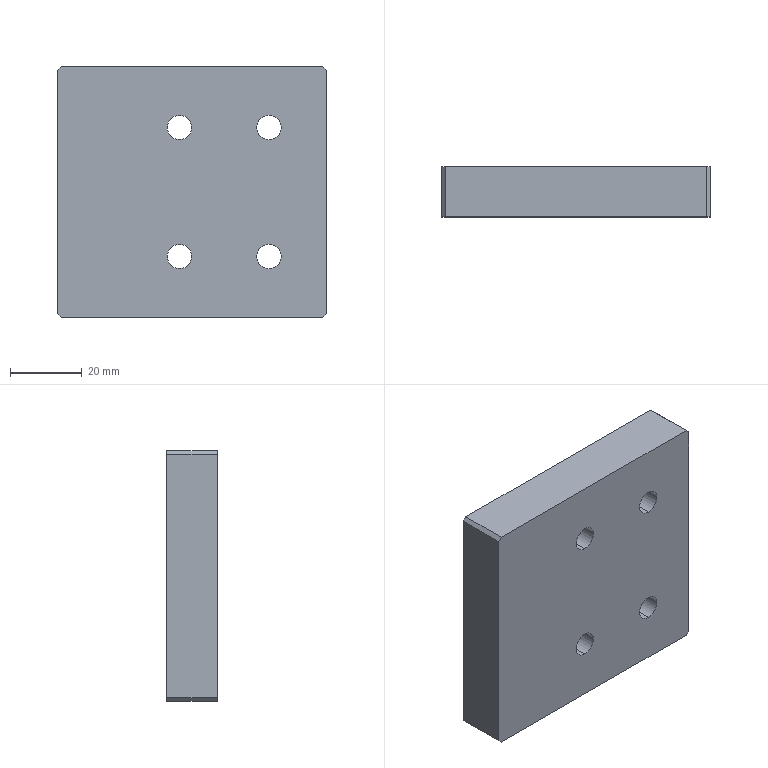Part | SolidWorks | features FlatPattern 1, HoleWzd 1, SMBaseFlange 1, SheetMetal 1 | 1 solid | 18 faces | box 75 x 14 x 70 mm | volume 71438 mm3 | plane 10 | cylinder 8 | commonest cylinder face diameters 6.8 x8
STEP:
#1=CARTESIAN_POINT('',(21.5,0.,-14.6));
#2=VERTEX_POINT('',#1);
#3=CARTESIAN_POINT('',(21.5,0.,-21.4));
#4=VERTEX_POINT('',#3);
#5=CARTESIAN_POINT('',(21.5,0.,-18.));
#6=DIRECTION('',(0.,-1.,0.));
#7=DIRECTION('',(0.,0.,-1.));
#8=AXIS2_PLACEMENT_3D('',#5,#6,#7);
#9=CIRCLE('',#8,3.4);
#10=EDGE_CURVE('',#2,#4,#9,.T.);
#11=ORIENTED_EDGE('',*,*,#10,.T.);
#12=CARTESIAN_POINT('',(21.5,14.,-21.4));
#13=VERTEX_POINT('',#12);
#14=CARTESIAN_POINT('',(21.5,14.,-21.4));
#15=DIRECTION('',(0.,1.,0.));
#16=VECTOR('',#15,1000.);
#17=LINE('',#14,#16);
#18=EDGE_CURVE('',#4,#13,#17,.T.);
#19=ORIENTED_EDGE('',*,*,#18,.T.);
#20=CARTESIAN_POINT('',(21.5,14.,-14.6));
#21=VERTEX_POINT('',#20);
#22=CARTESIAN_POINT('',(21.5,14.,-18.));
#23=DIRECTION('',(0.,1.,0.));
#24=DIRECTION('',(0.,0.,1.));
#25=AXIS2_PLACEMENT_3D('',#22,#23,#24);
#26=CIRCLE('',#25,3.4);
#27=EDGE_CURVE('',#13,#21,#26,.T.);
#28=ORIENTED_EDGE('',*,*,#27,.T.);
#29=CARTESIAN_POINT('',(21.5,14.,-14.6));
#30=DIRECTION('',(0.,1.,0.));
#31=VECTOR('',#30,1000.);
#32=LINE('',#29,#31);
#33=EDGE_CURVE('',#2,#21,#32,.T.);
#34=ORIENTED_EDGE('',*,*,#33,.F.);
#35=EDGE_LOOP('',(#11,#19,#28,#34));
#36=FACE_OUTER_BOUND('',#35,.T.);
#37=CARTESIAN_POINT('',(21.5,14.,-18.));
#38=DIRECTION('',(0.,1.,0.));
#39=DIRECTION('',(0.,0.,1.));
#40=AXIS2_PLACEMENT_3D('',#37,#38,#39);
#41=CYLINDRICAL_SURFACE('',#40,3.4);
#42=ADVANCED_FACE('',(#36),#41,.F.);
#43=CARTESIAN_POINT('',(-3.5,0.,-14.6));
#44=VERTEX_POINT('',#43);
#45=CARTESIAN_POINT('',(-3.5,0.,-21.4));
#46=VERTEX_POINT('',#45);
#47=CARTESIAN_POINT('',(-3.5,0.,-18.));
#48=DIRECTION('',(0.,-1.,0.));
#49=DIRECTION('',(0.,0.,-1.));
#50=AXIS2_PLACEMENT_3D('',#47,#48,#49);
#51=CIRCLE('',#50,3.4);
#52=EDGE_CURVE('',#44,#46,#51,.T.);
#53=ORIENTED_EDGE('',*,*,#52,.T.);
#54=CARTESIAN_POINT('',(-3.5,14.,-21.4));
#55=VERTEX_POINT('',#54);
#56=CARTESIAN_POINT('',(-3.5,14.,-21.4));
#57=DIRECTION('',(0.,1.,0.));
#58=VECTOR('',#57,1000.);
#59=LINE('',#56,#58);
#60=EDGE_CURVE('',#46,#55,#59,.T.);
#61=ORIENTED_EDGE('',*,*,#60,.T.);
#62=CARTESIAN_POINT('',(-3.5,14.,-14.6));
#63=VERTEX_POINT('',#62);
#64=CARTESIAN_POINT('',(-3.5,14.,-18.));
#65=DIRECTION('',(0.,1.,0.));
#66=DIRECTION('',(0.,0.,1.));
#67=AXIS2_PLACEMENT_3D('',#64,#65,#66);
#68=CIRCLE('',#67,3.4);
#69=EDGE_CURVE('',#55,#63,#68,.T.);
#70=ORIENTED_EDGE('',*,*,#69,.T.);
#71=CARTESIAN_POINT('',(-3.5,14.,-14.6));
#72=DIRECTION('',(0.,1.,0.));
#73=VECTOR('',#72,1000.);
#74=LINE('',#71,#73);
#75=EDGE_CURVE('',#44,#63,#74,.T.);
#76=ORIENTED_EDGE('',*,*,#75,.F.);
#77=EDGE_LOOP('',(#53,#61,#70,#76));
#78=FACE_OUTER_BOUND('',#77,.T.);
#79=CARTESIAN_POINT('',(-3.5,14.,-18.));
#80=DIRECTION('',(0.,1.,0.));
#81=DIRECTION('',(0.,0.,1.));
#82=AXIS2_PLACEMENT_3D('',#79,#80,#81);
#83=CYLINDRICAL_SURFACE('',#82,3.4);
#84=ADVANCED_FACE('',(#78),#83,.F.);
#85=CARTESIAN_POINT('',(-3.5,0.,21.4));
#86=VERTEX_POINT('',#85);
#87=CARTESIAN_POINT('',(-3.5,0.,14.6));
#88=VERTEX_POINT('',#87);
#89=CARTESIAN_POINT('',(-3.5,0.,18.));
#90=DIRECTION('',(0.,-1.,0.));
#91=DIRECTION('',(0.,0.,-1.));
#92=AXIS2_PLACEMENT_3D('',#89,#90,#91);
#93=CIRCLE('',#92,3.4);
#94=EDGE_CURVE('',#86,#88,#93,.T.);
#95=ORIENTED_EDGE('',*,*,#94,.T.);
#96=CARTESIAN_POINT('',(-3.5,14.,14.6));
#97=VERTEX_POINT('',#96);
#98=CARTESIAN_POINT('',(-3.5,14.,14.6));
#99=DIRECTION('',(0.,1.,0.));
#100=VECTOR('',#99,1000.);
#101=LINE('',#98,#100);
#102=EDGE_CURVE('',#88,#97,#101,.T.);
#103=ORIENTED_EDGE('',*,*,#102,.T.);
#104=CARTESIAN_POINT('',(-3.5,14.,21.4));
#105=VERTEX_POINT('',#104);
#106=CARTESIAN_POINT('',(-3.5,14.,18.));
#107=DIRECTION('',(0.,1.,0.));
#108=DIRECTION('',(0.,0.,1.));
#109=AXIS2_PLACEMENT_3D('',#106,#107,#108);
#110=CIRCLE('',#109,3.4);
#111=EDGE_CURVE('',#97,#105,#110,.T.);
#112=ORIENTED_EDGE('',*,*,#111,.T.);
#113=CARTESIAN_POINT('',(-3.5,14.,21.4));
#114=DIRECTION('',(0.,1.,0.));
#115=VECTOR('',#114,1000.);
#116=LINE('',#113,#115);
#117=EDGE_CURVE('',#86,#105,#116,.T.);
#118=ORIENTED_EDGE('',*,*,#117,.F.);
#119=EDGE_LOOP('',(#95,#103,#112,#118));
#120=FACE_OUTER_BOUND('',#119,.T.);
#121=CARTESIAN_POINT('',(-3.5,14.,18.));
#122=DIRECTION('',(0.,1.,0.));
#123=DIRECTION('',(0.,0.,1.));
#124=AXIS2_PLACEMENT_3D('',#121,#122,#123);
#125=CYLINDRICAL_SURFACE('',#124,3.4);
#126=ADVANCED_FACE('',(#120),#125,.F.);
#127=CARTESIAN_POINT('',(21.5,0.,21.4));
#128=VERTEX_POINT('',#127);
#129=CARTESIAN_POINT('',(21.5,0.,14.6));
#130=VERTEX_POINT('',#129);
#131=CARTESIAN_POINT('',(21.5,0.,18.));
#132=DIRECTION('',(0.,-1.,0.));
#133=DIRECTION('',(0.,0.,-1.));
#134=AXIS2_PLACEMENT_3D('',#131,#132,#133);
#135=CIRCLE('',#134,3.4);
#136=EDGE_CURVE('',#128,#130,#135,.T.);
#137=ORIENTED_EDGE('',*,*,#136,.T.);
#138=CARTESIAN_POINT('',(21.5,14.,14.6));
#139=VERTEX_POINT('',#138);
#140=CARTESIAN_POINT('',(21.5,14.,14.6));
#141=DIRECTION('',(0.,1.,0.));
#142=VECTOR('',#141,1000.);
#143=LINE('',#140,#142);
#144=EDGE_CURVE('',#130,#139,#143,.T.);
#145=ORIENTED_EDGE('',*,*,#144,.T.);
#146=CARTESIAN_POINT('',(21.5,14.,21.4));
#147=VERTEX_POINT('',#146);
#148=CARTESIAN_POINT('',(21.5,14.,18.));
#149=DIRECTION('',(0.,1.,0.));
#150=DIRECTION('',(0.,0.,1.));
#151=AXIS2_PLACEMENT_3D('',#148,#149,#150);
#152=CIRCLE('',#151,3.4);
#153=EDGE_CURVE('',#139,#147,#152,.T.);
#154=ORIENTED_EDGE('',*,*,#153,.T.);
#155=CARTESIAN_POINT('',(21.5,14.,21.4));
#156=DIRECTION('',(0.,1.,0.));
#157=VECTOR('',#156,1000.);
#158=LINE('',#155,#157);
#159=EDGE_CURVE('',#128,#147,#158,.T.);
#160=ORIENTED_EDGE('',*,*,#159,.F.);
#161=EDGE_LOOP('',(#137,#145,#154,#160));
#162=FACE_OUTER_BOUND('',#161,.T.);
#163=CARTESIAN_POINT('',(21.5,14.,18.));
#164=DIRECTION('',(0.,1.,0.));
#165=DIRECTION('',(0.,0.,1.));
#166=AXIS2_PLACEMENT_3D('',#163,#164,#165);
#167=CYLINDRICAL_SURFACE('',#166,3.4);
#168=ADVANCED_FACE('',(#162),#167,.F.);
#169=CARTESIAN_POINT('',(21.5,14.,-18.));
#170=DIRECTION('',(0.,1.,0.));
#171=DIRECTION('',(0.,0.,1.));
#172=AXIS2_PLACEMENT_3D('',#169,#170,#171);
#173=CIRCLE('',#172,3.4);
#174=EDGE_CURVE('',#21,#13,#173,.T.);
#175=ORIENTED_EDGE('',*,*,#174,.F.);
#176=ORIENTED_EDGE('',*,*,#27,.F.);
#177=EDGE_LOOP('',(#175,#176));
#178=FACE_BOUND('',#177,.T.);
#179=CARTESIAN_POINT('',(-3.5,14.,-18.));
#180=DIRECTION('',(0.,1.,0.));
#181=DIRECTION('',(0.,0.,1.));
#182=AXIS2_PLACEMENT_3D('',#179,#180,#181);
#183=CIRCLE('',#182,3.4);
#184=EDGE_CURVE('',#63,#55,#183,.T.);
#185=ORIENTED_EDGE('',*,*,#184,.F.);
#186=ORIENTED_EDGE('',*,*,#69,.F.);
#187=EDGE_LOOP('',(#185,#186));
#188=FACE_BOUND('',#187,.T.);
#189=CARTESIAN_POINT('',(-3.5,14.,18.));
#190=DIRECTION('',(0.,1.,0.));
#191=DIRECTION('',(0.,0.,1.));
#192=AXIS2_PLACEMENT_3D('',#189,#190,#191);
#193=CIRCLE('',#192,3.4);
#194=EDGE_CURVE('',#105,#97,#193,.T.);
#195=ORIENTED_EDGE('',*,*,#194,.F.);
#196=ORIENTED_EDGE('',*,*,#111,.F.);
#197=EDGE_LOOP('',(#195,#196));
#198=FACE_BOUND('',#197,.T.);
#199=CARTESIAN_POINT('',(21.5,14.,18.));
#200=DIRECTION('',(0.,1.,0.));
#201=DIRECTION('',(0.,0.,1.));
#202=AXIS2_PLACEMENT_3D('',#199,#200,#201);
#203=CIRCLE('',#202,3.4);
#204=EDGE_CURVE('',#147,#139,#203,.T.);
#205=ORIENTED_EDGE('',*,*,#204,.F.);
#206=ORIENTED_EDGE('',*,*,#153,.F.);
#207=EDGE_LOOP('',(#205,#206));
#208=FACE_BOUND('',#207,.T.);
#209=CARTESIAN_POINT('',(36.5,14.,-35.));
#210=VERTEX_POINT('',#209);
#211=CARTESIAN_POINT('',(-36.5,14.,-35.));
#212=VERTEX_POINT('',#211);
#213=CARTESIAN_POINT('',(-36.5,14.,-35.));
#214=DIRECTION('',(-1.,0.,0.));
#215=VECTOR('',#214,1000.);
#216=LINE('',#213,#215);
#217=EDGE_CURVE('',#210,#212,#216,.T.);
#218=ORIENTED_EDGE('',*,*,#217,.T.);
#219=CARTESIAN_POINT('',(-37.5,14.,-34.));
#220=VERTEX_POINT('',#219);
#221=CARTESIAN_POINT('',(-37.5,14.,-34.));
#222=DIRECTION('',(-0.7071,0.,0.7071));
#223=VECTOR('',#222,1000.);
#224=LINE('',#221,#223);
#225=EDGE_CURVE('',#212,#220,#224,.T.);
#226=ORIENTED_EDGE('',*,*,#225,.T.);
#227=CARTESIAN_POINT('',(-37.5,14.,34.));
#228=VERTEX_POINT('',#227);
#229=CARTESIAN_POINT('',(-37.5,14.,-34.));
#230=DIRECTION('',(0.,0.,1.));
#231=VECTOR('',#230,1000.);
#232=LINE('',#229,#231);
#233=EDGE_CURVE('',#220,#228,#232,.T.);
#234=ORIENTED_EDGE('',*,*,#233,.T.);
#235=CARTESIAN_POINT('',(-36.5,14.,35.));
#236=VERTEX_POINT('',#235);
#237=CARTESIAN_POINT('',(-37.5,14.,34.));
#238=DIRECTION('',(0.7071,0.,0.7071));
#239=VECTOR('',#238,1000.);
#240=LINE('',#237,#239);
#241=EDGE_CURVE('',#228,#236,#240,.T.);
#242=ORIENTED_EDGE('',*,*,#241,.T.);
#243=CARTESIAN_POINT('',(36.5,14.,35.));
#244=VERTEX_POINT('',#243);
#245=CARTESIAN_POINT('',(-36.5,14.,35.));
#246=DIRECTION('',(1.,0.,0.));
#247=VECTOR('',#246,1000.);
#248=LINE('',#245,#247);
#249=EDGE_CURVE('',#236,#244,#248,.T.);
#250=ORIENTED_EDGE('',*,*,#249,.T.);
#251=CARTESIAN_POINT('',(37.5,14.,34.));
#252=VERTEX_POINT('',#251);
#253=CARTESIAN_POINT('',(36.5,14.,35.));
#254=DIRECTION('',(0.7071,0.,-0.7071));
#255=VECTOR('',#254,1000.);
#256=LINE('',#253,#255);
#257=EDGE_CURVE('',#244,#252,#256,.T.);
#258=ORIENTED_EDGE('',*,*,#257,.T.);
#259=CARTESIAN_POINT('',(37.5,14.,-34.));
#260=VERTEX_POINT('',#259);
#261=CARTESIAN_POINT('',(37.5,14.,-34.));
#262=DIRECTION('',(0.,0.,-1.));
#263=VECTOR('',#262,1000.);
#264=LINE('',#261,#263);
#265=EDGE_CURVE('',#252,#260,#264,.T.);
#266=ORIENTED_EDGE('',*,*,#265,.T.);
#267=CARTESIAN_POINT('',(36.5,14.,-35.));
#268=DIRECTION('',(-0.7071,0.,-0.7071));
#269=VECTOR('',#268,1000.);
#270=LINE('',#267,#269);
#271=EDGE_CURVE('',#260,#210,#270,.T.);
#272=ORIENTED_EDGE('',*,*,#271,.T.);
#273=EDGE_LOOP('',(#218,#226,#234,#242,#250,#258,#266,#272));
#274=FACE_OUTER_BOUND('',#273,.T.);
#275=CARTESIAN_POINT('',(0.,14.,0.));
#276=DIRECTION('',(0.,-1.,0.));
#277=DIRECTION('',(0.,0.,-1.));
#278=AXIS2_PLACEMENT_3D('',#275,#276,#277);
#279=PLANE('',#278);
#280=ADVANCED_FACE('',(#178,#188,#198,#208,#274),#279,.F.);
#281=ORIENTED_EDGE('',*,*,#10,.F.);
#282=CARTESIAN_POINT('',(21.5,0.,-18.));
#283=DIRECTION('',(0.,-1.,0.));
#284=DIRECTION('',(0.,0.,-1.));
#285=AXIS2_PLACEMENT_3D('',#282,#283,#284);
#286=CIRCLE('',#285,3.4);
#287=EDGE_CURVE('',#4,#2,#286,.T.);
#288=ORIENTED_EDGE('',*,*,#287,.F.);
#289=EDGE_LOOP('',(#281,#288));
#290=FACE_BOUND('',#289,.T.);
#291=ORIENTED_EDGE('',*,*,#52,.F.);
#292=CARTESIAN_POINT('',(-3.5,0.,-18.));
#293=DIRECTION('',(0.,-1.,0.));
#294=DIRECTION('',(0.,0.,-1.));
#295=AXIS2_PLACEMENT_3D('',#292,#293,#294);
#296=CIRCLE('',#295,3.4);
#297=EDGE_CURVE('',#46,#44,#296,.T.);
#298=ORIENTED_EDGE('',*,*,#297,.F.);
#299=EDGE_LOOP('',(#291,#298));
#300=FACE_BOUND('',#299,.T.);
#301=ORIENTED_EDGE('',*,*,#94,.F.);
#302=CARTESIAN_POINT('',(-3.5,0.,18.));
#303=DIRECTION('',(0.,-1.,0.));
#304=DIRECTION('',(0.,0.,-1.));
#305=AXIS2_PLACEMENT_3D('',#302,#303,#304);
#306=CIRCLE('',#305,3.4);
#307=EDGE_CURVE('',#88,#86,#306,.T.);
#308=ORIENTED_EDGE('',*,*,#307,.F.);
#309=EDGE_LOOP('',(#301,#308));
#310=FACE_BOUND('',#309,.T.);
#311=ORIENTED_EDGE('',*,*,#136,.F.);
#312=CARTESIAN_POINT('',(21.5,0.,18.));
#313=DIRECTION('',(0.,-1.,0.));
#314=DIRECTION('',(0.,0.,-1.));
#315=AXIS2_PLACEMENT_3D('',#312,#313,#314);
#316=CIRCLE('',#315,3.4);
#317=EDGE_CURVE('',#130,#128,#316,.T.);
#318=ORIENTED_EDGE('',*,*,#317,.F.);
#319=EDGE_LOOP('',(#311,#318));
#320=FACE_BOUND('',#319,.T.);
#321=CARTESIAN_POINT('',(36.5,0.,-35.));
#322=VERTEX_POINT('',#321);
#323=CARTESIAN_POINT('',(-36.5,0.,-35.));
#324=VERTEX_POINT('',#323);
#325=CARTESIAN_POINT('',(-36.5,0.,-35.));
#326=DIRECTION('',(-1.,0.,0.));
#327=VECTOR('',#326,1000.);
#328=LINE('',#325,#327);
#329=EDGE_CURVE('',#322,#324,#328,.T.);
#330=ORIENTED_EDGE('',*,*,#329,.F.);
#331=CARTESIAN_POINT('',(37.5,0.,-34.));
#332=VERTEX_POINT('',#331);
#333=CARTESIAN_POINT('',(36.5,0.,-35.));
#334=DIRECTION('',(-0.7071,0.,-0.7071));
#335=VECTOR('',#334,1000.);
#336=LINE('',#333,#335);
#337=EDGE_CURVE('',#332,#322,#336,.T.);
#338=ORIENTED_EDGE('',*,*,#337,.F.);
#339=CARTESIAN_POINT('',(37.5,0.,34.));
#340=VERTEX_POINT('',#339);
#341=CARTESIAN_POINT('',(37.5,0.,-34.));
#342=DIRECTION('',(0.,0.,-1.));
#343=VECTOR('',#342,1000.);
#344=LINE('',#341,#343);
#345=EDGE_CURVE('',#340,#332,#344,.T.);
#346=ORIENTED_EDGE('',*,*,#345,.F.);
#347=CARTESIAN_POINT('',(36.5,0.,35.));
#348=VERTEX_POINT('',#347);
#349=CARTESIAN_POINT('',(36.5,0.,35.));
#350=DIRECTION('',(0.7071,0.,-0.7071));
#351=VECTOR('',#350,1000.);
#352=LINE('',#349,#351);
#353=EDGE_CURVE('',#348,#340,#352,.T.);
#354=ORIENTED_EDGE('',*,*,#353,.F.);
#355=CARTESIAN_POINT('',(-36.5,0.,35.));
#356=VERTEX_POINT('',#355);
#357=CARTESIAN_POINT('',(-36.5,0.,35.));
#358=DIRECTION('',(1.,0.,0.));
#359=VECTOR('',#358,1000.);
#360=LINE('',#357,#359);
#361=EDGE_CURVE('',#356,#348,#360,.T.);
#362=ORIENTED_EDGE('',*,*,#361,.F.);
#363=CARTESIAN_POINT('',(-37.5,0.,34.));
#364=VERTEX_POINT('',#363);
#365=CARTESIAN_POINT('',(-37.5,0.,34.));
#366=DIRECTION('',(0.7071,0.,0.7071));
#367=VECTOR('',#366,1000.);
#368=LINE('',#365,#367);
#369=EDGE_CURVE('',#364,#356,#368,.T.);
#370=ORIENTED_EDGE('',*,*,#369,.F.);
#371=CARTESIAN_POINT('',(-37.5,0.,-34.));
#372=VERTEX_POINT('',#371);
#373=CARTESIAN_POINT('',(-37.5,0.,-34.));
#374=DIRECTION('',(0.,0.,1.));
#375=VECTOR('',#374,1000.);
#376=LINE('',#373,#375);
#377=EDGE_CURVE('',#372,#364,#376,.T.);
#378=ORIENTED_EDGE('',*,*,#377,.F.);
#379=CARTESIAN_POINT('',(-37.5,0.,-34.));
#380=DIRECTION('',(-0.7071,0.,0.7071));
#381=VECTOR('',#380,1000.);
#382=LINE('',#379,#381);
#383=EDGE_CURVE('',#324,#372,#382,.T.);
#384=ORIENTED_EDGE('',*,*,#383,.F.);
#385=EDGE_LOOP('',(#330,#338,#346,#354,#362,#370,#378,#384));
#386=FACE_OUTER_BOUND('',#385,.T.);
#387=CARTESIAN_POINT('',(0.,0.,0.));
#388=DIRECTION('',(0.,-1.,0.));
#389=DIRECTION('',(0.,0.,-1.));
#390=AXIS2_PLACEMENT_3D('',#387,#388,#389);
#391=PLANE('',#390);
#392=ADVANCED_FACE('',(#290,#300,#310,#320,#386),#391,.T.);
#393=ORIENTED_EDGE('',*,*,#329,.T.);
#394=CARTESIAN_POINT('',(-36.5,14.,-35.));
#395=DIRECTION('',(0.,-1.,0.));
#396=VECTOR('',#395,1000.);
#397=LINE('',#394,#396);
#398=EDGE_CURVE('',#212,#324,#397,.T.);
#399=ORIENTED_EDGE('',*,*,#398,.F.);
#400=ORIENTED_EDGE('',*,*,#217,.F.);
#401=CARTESIAN_POINT('',(36.5,14.,-35.));
#402=DIRECTION('',(0.,-1.,0.));
#403=VECTOR('',#402,1000.);
#404=LINE('',#401,#403);
#405=EDGE_CURVE('',#210,#322,#404,.T.);
#406=ORIENTED_EDGE('',*,*,#405,.T.);
#407=EDGE_LOOP('',(#393,#399,#400,#406));
#408=FACE_OUTER_BOUND('',#407,.T.);
#409=CARTESIAN_POINT('',(-36.5,14.,-35.));
#410=DIRECTION('',(0.,0.,1.));
#411=DIRECTION('',(1.,0.,0.));
#412=AXIS2_PLACEMENT_3D('',#409,#410,#411);
#413=PLANE('',#412);
#414=ADVANCED_FACE('',(#408),#413,.F.);
#415=ORIENTED_EDGE('',*,*,#383,.T.);
#416=CARTESIAN_POINT('',(-37.5,14.,-34.));
#417=DIRECTION('',(0.,-1.,0.));
#418=VECTOR('',#417,1000.);
#419=LINE('',#416,#418);
#420=EDGE_CURVE('',#220,#372,#419,.T.);
#421=ORIENTED_EDGE('',*,*,#420,.F.);
#422=ORIENTED_EDGE('',*,*,#225,.F.);
#423=ORIENTED_EDGE('',*,*,#398,.T.);
#424=EDGE_LOOP('',(#415,#421,#422,#423));
#425=FACE_OUTER_BOUND('',#424,.T.);
#426=CARTESIAN_POINT('',(-37.5,14.,-34.));
#427=DIRECTION('',(0.7071,0.,0.7071));
#428=DIRECTION('',(0.7071,0.,-0.7071));
#429=AXIS2_PLACEMENT_3D('',#426,#427,#428);
#430=PLANE('',#429);
#431=ADVANCED_FACE('',(#425),#430,.F.);
#432=ORIENTED_EDGE('',*,*,#377,.T.);
#433=CARTESIAN_POINT('',(-37.5,14.,34.));
#434=DIRECTION('',(0.,-1.,0.));
#435=VECTOR('',#434,1000.);
#436=LINE('',#433,#435);
#437=EDGE_CURVE('',#228,#364,#436,.T.);
#438=ORIENTED_EDGE('',*,*,#437,.F.);
#439=ORIENTED_EDGE('',*,*,#233,.F.);
#440=ORIENTED_EDGE('',*,*,#420,.T.);
#441=EDGE_LOOP('',(#432,#438,#439,#440));
#442=FACE_OUTER_BOUND('',#441,.T.);
#443=CARTESIAN_POINT('',(-37.5,14.,-34.));
#444=DIRECTION('',(1.,0.,0.));
#445=DIRECTION('',(0.,0.,-1.));
#446=AXIS2_PLACEMENT_3D('',#443,#444,#445);
#447=PLANE('',#446);
#448=ADVANCED_FACE('',(#442),#447,.F.);
#449=ORIENTED_EDGE('',*,*,#369,.T.);
#450=CARTESIAN_POINT('',(-36.5,14.,35.));
#451=DIRECTION('',(0.,-1.,0.));
#452=VECTOR('',#451,1000.);
#453=LINE('',#450,#452);
#454=EDGE_CURVE('',#236,#356,#453,.T.);
#455=ORIENTED_EDGE('',*,*,#454,.F.);
#456=ORIENTED_EDGE('',*,*,#241,.F.);
#457=ORIENTED_EDGE('',*,*,#437,.T.);
#458=EDGE_LOOP('',(#449,#455,#456,#457));
#459=FACE_OUTER_BOUND('',#458,.T.);
#460=CARTESIAN_POINT('',(-37.5,14.,34.));
#461=DIRECTION('',(0.7071,0.,-0.7071));
#462=DIRECTION('',(-0.7071,0.,-0.7071));
#463=AXIS2_PLACEMENT_3D('',#460,#461,#462);
#464=PLANE('',#463);
#465=ADVANCED_FACE('',(#459),#464,.F.);
#466=ORIENTED_EDGE('',*,*,#361,.T.);
#467=CARTESIAN_POINT('',(36.5,14.,35.));
#468=DIRECTION('',(0.,-1.,0.));
#469=VECTOR('',#468,1000.);
#470=LINE('',#467,#469);
#471=EDGE_CURVE('',#244,#348,#470,.T.);
#472=ORIENTED_EDGE('',*,*,#471,.F.);
#473=ORIENTED_EDGE('',*,*,#249,.F.);
#474=ORIENTED_EDGE('',*,*,#454,.T.);
#475=EDGE_LOOP('',(#466,#472,#473,#474));
#476=FACE_OUTER_BOUND('',#475,.T.);
#477=CARTESIAN_POINT('',(-36.5,14.,35.));
#478=DIRECTION('',(0.,0.,-1.));
#479=DIRECTION('',(-1.,0.,0.));
#480=AXIS2_PLACEMENT_3D('',#477,#478,#479);
#481=PLANE('',#480);
#482=ADVANCED_FACE('',(#476),#481,.F.);
#483=ORIENTED_EDGE('',*,*,#353,.T.);
#484=CARTESIAN_POINT('',(37.5,14.,34.));
#485=DIRECTION('',(0.,-1.,0.));
#486=VECTOR('',#485,1000.);
#487=LINE('',#484,#486);
#488=EDGE_CURVE('',#252,#340,#487,.T.);
#489=ORIENTED_EDGE('',*,*,#488,.F.);
#490=ORIENTED_EDGE('',*,*,#257,.F.);
#491=ORIENTED_EDGE('',*,*,#471,.T.);
#492=EDGE_LOOP('',(#483,#489,#490,#491));
#493=FACE_OUTER_BOUND('',#492,.T.);
#494=CARTESIAN_POINT('',(36.5,14.,35.));
#495=DIRECTION('',(-0.7071,0.,-0.7071));
#496=DIRECTION('',(-0.7071,0.,0.7071));
#497=AXIS2_PLACEMENT_3D('',#494,#495,#496);
#498=PLANE('',#497);
#499=ADVANCED_FACE('',(#493),#498,.F.);
#500=ORIENTED_EDGE('',*,*,#345,.T.);
#501=CARTESIAN_POINT('',(37.5,14.,-34.));
#502=DIRECTION('',(0.,-1.,0.));
#503=VECTOR('',#502,1000.);
#504=LINE('',#501,#503);
#505=EDGE_CURVE('',#260,#332,#504,.T.);
#506=ORIENTED_EDGE('',*,*,#505,.F.);
#507=ORIENTED_EDGE('',*,*,#265,.F.);
#508=ORIENTED_EDGE('',*,*,#488,.T.);
#509=EDGE_LOOP('',(#500,#506,#507,#508));
#510=FACE_OUTER_BOUND('',#509,.T.);
#511=CARTESIAN_POINT('',(37.5,14.,-34.));
#512=DIRECTION('',(-1.,0.,0.));
#513=DIRECTION('',(0.,0.,1.));
#514=AXIS2_PLACEMENT_3D('',#511,#512,#513);
#515=PLANE('',#514);
#516=ADVANCED_FACE('',(#510),#515,.F.);
#517=ORIENTED_EDGE('',*,*,#337,.T.);
#518=ORIENTED_EDGE('',*,*,#405,.F.);
#519=ORIENTED_EDGE('',*,*,#271,.F.);
#520=ORIENTED_EDGE('',*,*,#505,.T.);
#521=EDGE_LOOP('',(#517,#518,#519,#520));
#522=FACE_OUTER_BOUND('',#521,.T.);
#523=CARTESIAN_POINT('',(36.5,14.,-35.));
#524=DIRECTION('',(-0.7071,0.,0.7071));
#525=DIRECTION('',(0.7071,0.,0.7071));
#526=AXIS2_PLACEMENT_3D('',#523,#524,#525);
#527=PLANE('',#526);
#528=ADVANCED_FACE('',(#522),#527,.F.);
#529=ORIENTED_EDGE('',*,*,#144,.F.);
#530=ORIENTED_EDGE('',*,*,#317,.T.);
#531=ORIENTED_EDGE('',*,*,#159,.T.);
#532=ORIENTED_EDGE('',*,*,#204,.T.);
#533=EDGE_LOOP('',(#529,#530,#531,#532));
#534=FACE_OUTER_BOUND('',#533,.T.);
#535=CARTESIAN_POINT('',(21.5,14.,18.));
#536=DIRECTION('',(0.,1.,0.));
#537=DIRECTION('',(0.,0.,1.));
#538=AXIS2_PLACEMENT_3D('',#535,#536,#537);
#539=CYLINDRICAL_SURFACE('',#538,3.4);
#540=ADVANCED_FACE('',(#534),#539,.F.);
#541=ORIENTED_EDGE('',*,*,#102,.F.);
#542=ORIENTED_EDGE('',*,*,#307,.T.);
#543=ORIENTED_EDGE('',*,*,#117,.T.);
#544=ORIENTED_EDGE('',*,*,#194,.T.);
#545=EDGE_LOOP('',(#541,#542,#543,#544));
#546=FACE_OUTER_BOUND('',#545,.T.);
#547=CARTESIAN_POINT('',(-3.5,14.,18.));
#548=DIRECTION('',(0.,1.,0.));
#549=DIRECTION('',(0.,0.,1.));
#550=AXIS2_PLACEMENT_3D('',#547,#548,#549);
#551=CYLINDRICAL_SURFACE('',#550,3.4);
#552=ADVANCED_FACE('',(#546),#551,.F.);
#553=ORIENTED_EDGE('',*,*,#60,.F.);
#554=ORIENTED_EDGE('',*,*,#297,.T.);
#555=ORIENTED_EDGE('',*,*,#75,.T.);
#556=ORIENTED_EDGE('',*,*,#184,.T.);
#557=EDGE_LOOP('',(#553,#554,#555,#556));
#558=FACE_OUTER_BOUND('',#557,.T.);
#559=CARTESIAN_POINT('',(-3.5,14.,-18.));
#560=DIRECTION('',(0.,1.,0.));
#561=DIRECTION('',(0.,0.,1.));
#562=AXIS2_PLACEMENT_3D('',#559,#560,#561);
#563=CYLINDRICAL_SURFACE('',#562,3.4);
#564=ADVANCED_FACE('',(#558),#563,.F.);
#565=ORIENTED_EDGE('',*,*,#18,.F.);
#566=ORIENTED_EDGE('',*,*,#287,.T.);
#567=ORIENTED_EDGE('',*,*,#33,.T.);
#568=ORIENTED_EDGE('',*,*,#174,.T.);
#569=EDGE_LOOP('',(#565,#566,#567,#568));
#570=FACE_OUTER_BOUND('',#569,.T.);
#571=CARTESIAN_POINT('',(21.5,14.,-18.));
#572=DIRECTION('',(0.,1.,0.));
#573=DIRECTION('',(0.,0.,1.));
#574=AXIS2_PLACEMENT_3D('',#571,#572,#573);
#575=CYLINDRICAL_SURFACE('',#574,3.4);
#576=ADVANCED_FACE('',(#570),#575,.F.);
#577=CLOSED_SHELL('',(#42,#84,#126,#168,#280,#392,#414,#431,#448,#465,#482,#499,#516,#528,#540,#552,#564,#576));
#578=MANIFOLD_SOLID_BREP('',#577);
#579=CARTESIAN_POINT('',(0.,0.,0.));
#580=DIRECTION('',(0.,0.,1.));
#581=DIRECTION('',(1.,0.,0.));
#582=AXIS2_PLACEMENT_3D('',#579,#580,#581);
#583=(LENGTH_UNIT()NAMED_UNIT(*)SI_UNIT(.MILLI.,.METRE.));
#584=UNCERTAINTY_MEASURE_WITH_UNIT(LENGTH_MEASURE(0.00001),#583,'','');
#585=(NAMED_UNIT(*)PLANE_ANGLE_UNIT()SI_UNIT($,.RADIAN.));
#586=(NAMED_UNIT(*)SI_UNIT($,.STERADIAN.)SOLID_ANGLE_UNIT());
#587=(GEOMETRIC_REPRESENTATION_CONTEXT(3)GLOBAL_UNCERTAINTY_ASSIGNED_CONTEXT((#584))GLOBAL_UNIT_ASSIGNED_CONTEXT((#583,#585,#586))REPRESENTATION_CONTEXT('',''));
#588=ADVANCED_BREP_SHAPE_REPRESENTATION('',(#578,#582),#587);